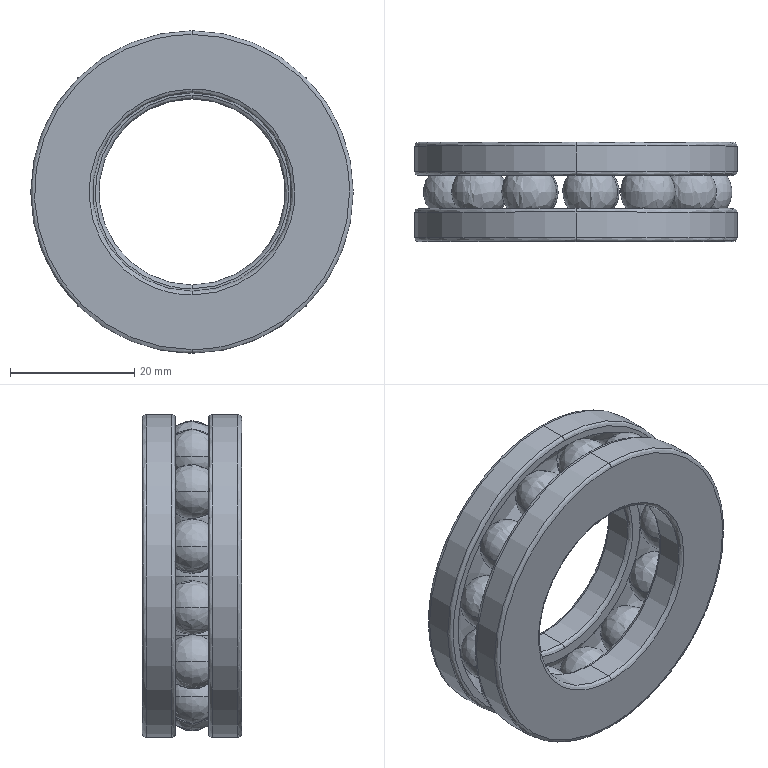Part | SolidWorks | features BaseBody 1 | 1 solid | 84 faces | box 52 x 16 x 52 mm | volume 16958 mm3 | spline 70 | cylinder 8 | plane 6 | commonest cylinder face diameters 52 x4 30 x2 32 x2